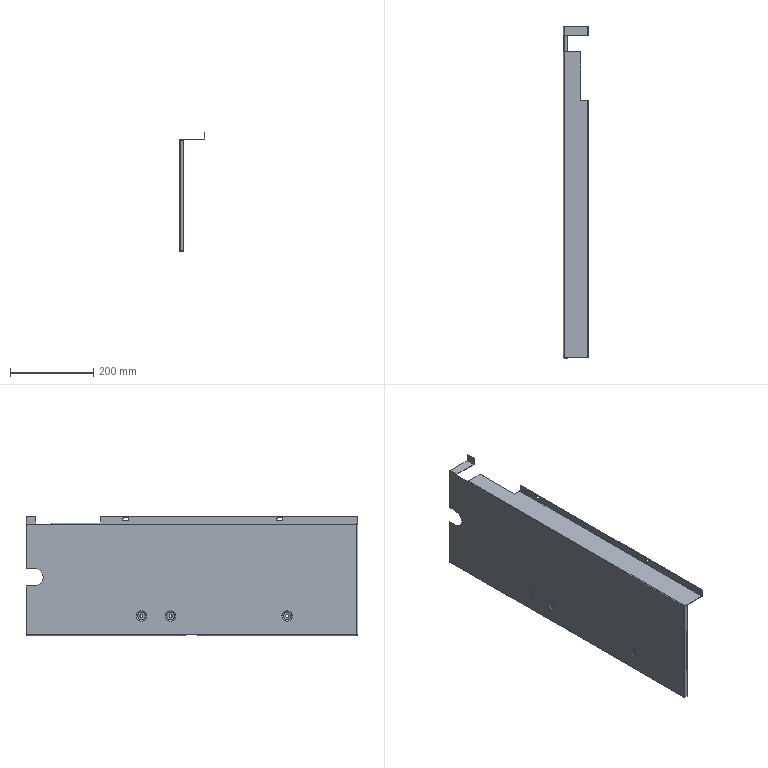Part | STEP file | 1 solid | 130 faces | box 62 x 797 x 286 mm | volume 329890 mm3 | plane 73 | cylinder 33 | torus 24 | commonest cylinder face diameters 7 x10 20 x6 22.4 x6 2 x5 4.4 x5 42 x1